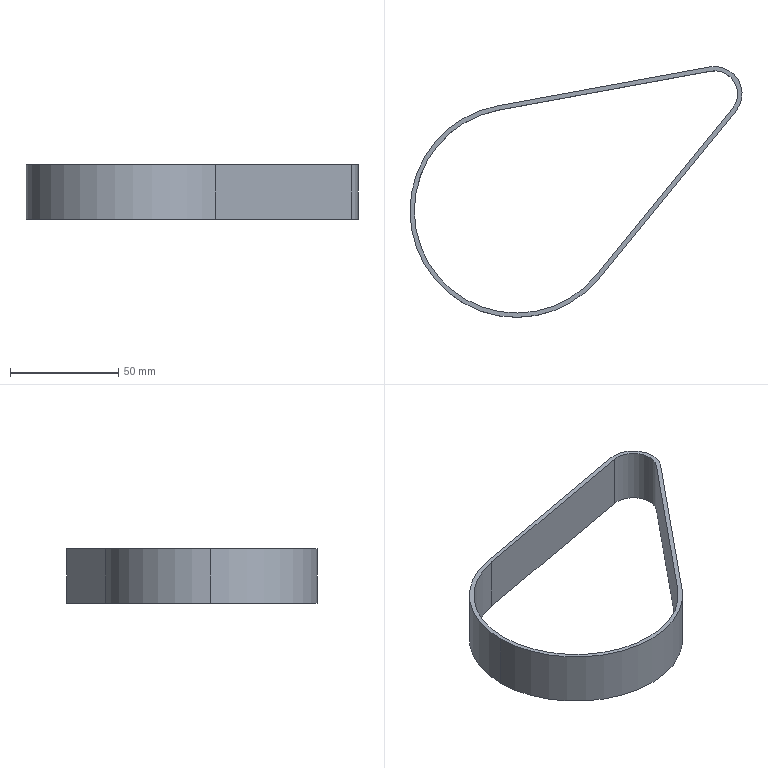Part | SolidWorks | features BaseBody 1 | 1 solid | 12 faces | box 153.425 x 115.925 x 25 mm | volume 20675 mm3 | plane 6 | cylinder 6 | commonest cylinder face diameters 94.53 x2 98.53 x2 21.32 x1 25.32 x1
STEP:
#1=CARTESIAN_POINT('',(-10.423,64.485,-12.5));
#2=VERTEX_POINT('',#1);
#3=CARTESIAN_POINT('',(-108.528,46.489,-12.5));
#4=VERTEX_POINT('',#3);
#5=CARTESIAN_POINT('',(-108.528,46.489,-12.5));
#6=DIRECTION('',(-0.9836,-0.1804,0.));
#7=VECTOR('',#6,1000.);
#8=LINE('',#5,#7);
#9=EDGE_CURVE('',#2,#4,#8,.T.);
#10=ORIENTED_EDGE('',*,*,#9,.F.);
#11=CARTESIAN_POINT('',(-10.423,64.485,12.5));
#12=VERTEX_POINT('',#11);
#13=CARTESIAN_POINT('',(-10.423,64.485,12.5));
#14=DIRECTION('',(0.,0.,-1.));
#15=VECTOR('',#14,1000.);
#16=LINE('',#13,#15);
#17=EDGE_CURVE('',#12,#2,#16,.T.);
#18=ORIENTED_EDGE('',*,*,#17,.F.);
#19=CARTESIAN_POINT('',(-108.528,46.489,12.5));
#20=VERTEX_POINT('',#19);
#21=CARTESIAN_POINT('',(-108.528,46.489,12.5));
#22=DIRECTION('',(-0.9836,-0.1804,0.));
#23=VECTOR('',#22,1000.);
#24=LINE('',#21,#23);
#25=EDGE_CURVE('',#12,#20,#24,.T.);
#26=ORIENTED_EDGE('',*,*,#25,.T.);
#27=CARTESIAN_POINT('',(-108.528,46.489,12.5));
#28=DIRECTION('',(0.,0.,-1.));
#29=VECTOR('',#28,1000.);
#30=LINE('',#27,#29);
#31=EDGE_CURVE('',#20,#4,#30,.T.);
#32=ORIENTED_EDGE('',*,*,#31,.T.);
#33=EDGE_LOOP('',(#10,#18,#26,#32));
#34=FACE_OUTER_BOUND('',#33,.T.);
#35=CARTESIAN_POINT('',(-108.528,46.489,12.5));
#36=DIRECTION('',(0.1804,-0.9836,0.));
#37=DIRECTION('',(0.,0.,-1.));
#38=AXIS2_PLACEMENT_3D('',#35,#36,#37);
#39=PLANE('',#38);
#40=ADVANCED_FACE('',(#34),#39,.T.);
#41=CARTESIAN_POINT('',(-0.2508,47.248,-12.5));
#42=VERTEX_POINT('',#41);
#43=CARTESIAN_POINT('',(-8.5,54.,-12.5));
#44=DIRECTION('',(0.,0.,1.));
#45=DIRECTION('',(-1.,0.,0.));
#46=AXIS2_PLACEMENT_3D('',#43,#44,#45);
#47=CIRCLE('',#46,10.66);
#48=EDGE_CURVE('',#42,#2,#47,.T.);
#49=ORIENTED_EDGE('',*,*,#48,.F.);
#50=CARTESIAN_POINT('',(-0.2508,47.248,12.5));
#51=VERTEX_POINT('',#50);
#52=CARTESIAN_POINT('',(-0.2508,47.248,12.5));
#53=DIRECTION('',(0.,0.,-1.));
#54=VECTOR('',#53,1000.);
#55=LINE('',#52,#54);
#56=EDGE_CURVE('',#51,#42,#55,.T.);
#57=ORIENTED_EDGE('',*,*,#56,.F.);
#58=CARTESIAN_POINT('',(-8.5,54.,12.5));
#59=DIRECTION('',(0.,0.,1.));
#60=DIRECTION('',(-1.,0.,0.));
#61=AXIS2_PLACEMENT_3D('',#58,#59,#60);
#62=CIRCLE('',#61,10.66);
#63=EDGE_CURVE('',#51,#12,#62,.T.);
#64=ORIENTED_EDGE('',*,*,#63,.T.);
#65=ORIENTED_EDGE('',*,*,#17,.T.);
#66=EDGE_LOOP('',(#49,#57,#64,#65));
#67=FACE_OUTER_BOUND('',#66,.T.);
#68=CARTESIAN_POINT('',(-8.5,54.,12.5));
#69=DIRECTION('',(0.,0.,-1.));
#70=DIRECTION('',(-1.,0.,0.));
#71=AXIS2_PLACEMENT_3D('',#68,#69,#70);
#72=CYLINDRICAL_SURFACE('',#71,10.66);
#73=ADVANCED_FACE('',(#67),#72,.F.);
#74=CARTESIAN_POINT('',(-63.424,-29.936,-12.5));
#75=VERTEX_POINT('',#74);
#76=CARTESIAN_POINT('',(-0.2508,47.248,-12.5));
#77=DIRECTION('',(0.6334,0.7738,0.));
#78=VECTOR('',#77,1000.);
#79=LINE('',#76,#78);
#80=EDGE_CURVE('',#75,#42,#79,.T.);
#81=ORIENTED_EDGE('',*,*,#80,.F.);
#82=CARTESIAN_POINT('',(-63.424,-29.936,12.5));
#83=VERTEX_POINT('',#82);
#84=CARTESIAN_POINT('',(-63.424,-29.936,12.5));
#85=DIRECTION('',(0.,0.,-1.));
#86=VECTOR('',#85,1000.);
#87=LINE('',#84,#86);
#88=EDGE_CURVE('',#83,#75,#87,.T.);
#89=ORIENTED_EDGE('',*,*,#88,.F.);
#90=CARTESIAN_POINT('',(-0.2508,47.248,12.5));
#91=DIRECTION('',(0.6334,0.7738,0.));
#92=VECTOR('',#91,1000.);
#93=LINE('',#90,#92);
#94=EDGE_CURVE('',#83,#51,#93,.T.);
#95=ORIENTED_EDGE('',*,*,#94,.T.);
#96=ORIENTED_EDGE('',*,*,#56,.T.);
#97=EDGE_LOOP('',(#81,#89,#95,#96));
#98=FACE_OUTER_BOUND('',#97,.T.);
#99=CARTESIAN_POINT('',(-0.2508,47.248,12.5));
#100=DIRECTION('',(-0.7738,0.6334,0.));
#101=DIRECTION('',(0.,0.,1.));
#102=AXIS2_PLACEMENT_3D('',#99,#100,#101);
#103=PLANE('',#102);
#104=ADVANCED_FACE('',(#98),#103,.T.);
#105=CARTESIAN_POINT('',(-147.265,0.,12.5));
#106=VERTEX_POINT('',#105);
#107=CARTESIAN_POINT('',(-147.265,0.,-12.5));
#108=VERTEX_POINT('',#107);
#109=CARTESIAN_POINT('',(-147.265,0.,12.5));
#110=DIRECTION('',(0.,0.,-1.));
#111=VECTOR('',#110,1000.);
#112=LINE('',#109,#111);
#113=EDGE_CURVE('',#106,#108,#112,.T.);
#114=ORIENTED_EDGE('',*,*,#113,.F.);
#115=CARTESIAN_POINT('',(-100.,0.,12.5));
#116=DIRECTION('',(0.,0.,1.));
#117=DIRECTION('',(-1.,0.,0.));
#118=AXIS2_PLACEMENT_3D('',#115,#116,#117);
#119=CIRCLE('',#118,47.265);
#120=EDGE_CURVE('',#106,#83,#119,.T.);
#121=ORIENTED_EDGE('',*,*,#120,.T.);
#122=ORIENTED_EDGE('',*,*,#88,.T.);
#123=CARTESIAN_POINT('',(-100.,0.,-12.5));
#124=DIRECTION('',(0.,0.,1.));
#125=DIRECTION('',(-1.,0.,0.));
#126=AXIS2_PLACEMENT_3D('',#123,#124,#125);
#127=CIRCLE('',#126,47.265);
#128=EDGE_CURVE('',#108,#75,#127,.T.);
#129=ORIENTED_EDGE('',*,*,#128,.F.);
#130=EDGE_LOOP('',(#114,#121,#122,#129));
#131=FACE_OUTER_BOUND('',#130,.T.);
#132=CARTESIAN_POINT('',(-100.,0.,12.5));
#133=DIRECTION('',(0.,0.,-1.));
#134=DIRECTION('',(-1.,0.,0.));
#135=AXIS2_PLACEMENT_3D('',#132,#133,#134);
#136=CYLINDRICAL_SURFACE('',#135,47.265);
#137=ADVANCED_FACE('',(#131),#136,.F.);
#138=CARTESIAN_POINT('',(-10.784,66.452,-12.5));
#139=VERTEX_POINT('',#138);
#140=CARTESIAN_POINT('',(-108.889,48.457,-12.5));
#141=VERTEX_POINT('',#140);
#142=CARTESIAN_POINT('',(-108.889,48.457,-12.5));
#143=DIRECTION('',(-0.9836,-0.1804,0.));
#144=VECTOR('',#143,1000.);
#145=LINE('',#142,#144);
#146=EDGE_CURVE('',#139,#141,#145,.T.);
#147=ORIENTED_EDGE('',*,*,#146,.T.);
#148=CARTESIAN_POINT('',(-108.889,48.457,12.5));
#149=VERTEX_POINT('',#148);
#150=CARTESIAN_POINT('',(-108.889,48.457,12.5));
#151=DIRECTION('',(0.,0.,-1.));
#152=VECTOR('',#151,1000.);
#153=LINE('',#150,#152);
#154=EDGE_CURVE('',#149,#141,#153,.T.);
#155=ORIENTED_EDGE('',*,*,#154,.F.);
#156=CARTESIAN_POINT('',(-10.784,66.452,12.5));
#157=VERTEX_POINT('',#156);
#158=CARTESIAN_POINT('',(-108.889,48.457,12.5));
#159=DIRECTION('',(-0.9836,-0.1804,0.));
#160=VECTOR('',#159,1000.);
#161=LINE('',#158,#160);
#162=EDGE_CURVE('',#157,#149,#161,.T.);
#163=ORIENTED_EDGE('',*,*,#162,.F.);
#164=CARTESIAN_POINT('',(-10.784,66.452,12.5));
#165=DIRECTION('',(0.,0.,-1.));
#166=VECTOR('',#165,1000.);
#167=LINE('',#164,#166);
#168=EDGE_CURVE('',#157,#139,#167,.T.);
#169=ORIENTED_EDGE('',*,*,#168,.T.);
#170=EDGE_LOOP('',(#147,#155,#163,#169));
#171=FACE_OUTER_BOUND('',#170,.T.);
#172=CARTESIAN_POINT('',(-108.889,48.457,12.5));
#173=DIRECTION('',(0.1804,-0.9836,0.));
#174=DIRECTION('',(0.,0.,-1.));
#175=AXIS2_PLACEMENT_3D('',#172,#173,#174);
#176=PLANE('',#175);
#177=ADVANCED_FACE('',(#171),#176,.F.);
#178=CARTESIAN_POINT('',(1.297,45.982,-12.5));
#179=VERTEX_POINT('',#178);
#180=CARTESIAN_POINT('',(-8.5,54.,-12.5));
#181=DIRECTION('',(0.,0.,1.));
#182=DIRECTION('',(-1.,0.,0.));
#183=AXIS2_PLACEMENT_3D('',#180,#181,#182);
#184=CIRCLE('',#183,12.66);
#185=EDGE_CURVE('',#179,#139,#184,.T.);
#186=ORIENTED_EDGE('',*,*,#185,.T.);
#187=ORIENTED_EDGE('',*,*,#168,.F.);
#188=CARTESIAN_POINT('',(1.297,45.982,12.5));
#189=VERTEX_POINT('',#188);
#190=CARTESIAN_POINT('',(-8.5,54.,12.5));
#191=DIRECTION('',(0.,0.,1.));
#192=DIRECTION('',(-1.,0.,0.));
#193=AXIS2_PLACEMENT_3D('',#190,#191,#192);
#194=CIRCLE('',#193,12.66);
#195=EDGE_CURVE('',#189,#157,#194,.T.);
#196=ORIENTED_EDGE('',*,*,#195,.F.);
#197=CARTESIAN_POINT('',(1.297,45.982,12.5));
#198=DIRECTION('',(0.,0.,-1.));
#199=VECTOR('',#198,1000.);
#200=LINE('',#197,#199);
#201=EDGE_CURVE('',#189,#179,#200,.T.);
#202=ORIENTED_EDGE('',*,*,#201,.T.);
#203=EDGE_LOOP('',(#186,#187,#196,#202));
#204=FACE_OUTER_BOUND('',#203,.T.);
#205=CARTESIAN_POINT('',(-8.5,54.,12.5));
#206=DIRECTION('',(0.,0.,-1.));
#207=DIRECTION('',(-1.,0.,0.));
#208=AXIS2_PLACEMENT_3D('',#205,#206,#207);
#209=CYLINDRICAL_SURFACE('',#208,12.66);
#210=ADVANCED_FACE('',(#204),#209,.T.);
#211=CARTESIAN_POINT('',(-61.876,-31.203,-12.5));
#212=VERTEX_POINT('',#211);
#213=CARTESIAN_POINT('',(-61.876,-31.203,-12.5));
#214=DIRECTION('',(0.6334,0.7738,0.));
#215=VECTOR('',#214,1000.);
#216=LINE('',#213,#215);
#217=EDGE_CURVE('',#212,#179,#216,.T.);
#218=ORIENTED_EDGE('',*,*,#217,.T.);
#219=ORIENTED_EDGE('',*,*,#201,.F.);
#220=CARTESIAN_POINT('',(-61.876,-31.203,12.5));
#221=VERTEX_POINT('',#220);
#222=CARTESIAN_POINT('',(-61.876,-31.203,12.5));
#223=DIRECTION('',(0.6334,0.7738,0.));
#224=VECTOR('',#223,1000.);
#225=LINE('',#222,#224);
#226=EDGE_CURVE('',#221,#189,#225,.T.);
#227=ORIENTED_EDGE('',*,*,#226,.F.);
#228=CARTESIAN_POINT('',(-61.876,-31.203,12.5));
#229=DIRECTION('',(0.,0.,-1.));
#230=VECTOR('',#229,1000.);
#231=LINE('',#228,#230);
#232=EDGE_CURVE('',#221,#212,#231,.T.);
#233=ORIENTED_EDGE('',*,*,#232,.T.);
#234=EDGE_LOOP('',(#218,#219,#227,#233));
#235=FACE_OUTER_BOUND('',#234,.T.);
#236=CARTESIAN_POINT('',(-61.876,-31.203,12.5));
#237=DIRECTION('',(-0.7738,0.6334,0.));
#238=DIRECTION('',(0.,0.,1.));
#239=AXIS2_PLACEMENT_3D('',#236,#237,#238);
#240=PLANE('',#239);
#241=ADVANCED_FACE('',(#235),#240,.F.);
#242=CARTESIAN_POINT('',(-149.265,0.,12.5));
#243=VERTEX_POINT('',#242);
#244=CARTESIAN_POINT('',(-149.265,0.,-12.5));
#245=VERTEX_POINT('',#244);
#246=CARTESIAN_POINT('',(-149.265,0.,12.5));
#247=DIRECTION('',(0.,0.,-1.));
#248=VECTOR('',#247,1000.);
#249=LINE('',#246,#248);
#250=EDGE_CURVE('',#243,#245,#249,.T.);
#251=ORIENTED_EDGE('',*,*,#250,.F.);
#252=CARTESIAN_POINT('',(-100.,0.,12.5));
#253=DIRECTION('',(0.,0.,1.));
#254=DIRECTION('',(-1.,0.,0.));
#255=AXIS2_PLACEMENT_3D('',#252,#253,#254);
#256=CIRCLE('',#255,49.265);
#257=EDGE_CURVE('',#149,#243,#256,.T.);
#258=ORIENTED_EDGE('',*,*,#257,.F.);
#259=ORIENTED_EDGE('',*,*,#154,.T.);
#260=CARTESIAN_POINT('',(-100.,0.,-12.5));
#261=DIRECTION('',(0.,0.,1.));
#262=DIRECTION('',(-1.,0.,0.));
#263=AXIS2_PLACEMENT_3D('',#260,#261,#262);
#264=CIRCLE('',#263,49.265);
#265=EDGE_CURVE('',#141,#245,#264,.T.);
#266=ORIENTED_EDGE('',*,*,#265,.T.);
#267=EDGE_LOOP('',(#251,#258,#259,#266));
#268=FACE_OUTER_BOUND('',#267,.T.);
#269=CARTESIAN_POINT('',(-100.,0.,12.5));
#270=DIRECTION('',(0.,0.,-1.));
#271=DIRECTION('',(-1.,0.,0.));
#272=AXIS2_PLACEMENT_3D('',#269,#270,#271);
#273=CYLINDRICAL_SURFACE('',#272,49.265);
#274=ADVANCED_FACE('',(#268),#273,.T.);
#275=ORIENTED_EDGE('',*,*,#9,.T.);
#276=CARTESIAN_POINT('',(-100.,0.,-12.5));
#277=DIRECTION('',(0.,0.,1.));
#278=DIRECTION('',(-1.,0.,0.));
#279=AXIS2_PLACEMENT_3D('',#276,#277,#278);
#280=CIRCLE('',#279,47.265);
#281=EDGE_CURVE('',#4,#108,#280,.T.);
#282=ORIENTED_EDGE('',*,*,#281,.T.);
#283=ORIENTED_EDGE('',*,*,#128,.T.);
#284=ORIENTED_EDGE('',*,*,#80,.T.);
#285=ORIENTED_EDGE('',*,*,#48,.T.);
#286=EDGE_LOOP('',(#275,#282,#283,#284,#285));
#287=FACE_BOUND('',#286,.T.);
#288=ORIENTED_EDGE('',*,*,#265,.F.);
#289=ORIENTED_EDGE('',*,*,#146,.F.);
#290=ORIENTED_EDGE('',*,*,#185,.F.);
#291=ORIENTED_EDGE('',*,*,#217,.F.);
#292=CARTESIAN_POINT('',(-100.,0.,-12.5));
#293=DIRECTION('',(0.,0.,1.));
#294=DIRECTION('',(-1.,0.,0.));
#295=AXIS2_PLACEMENT_3D('',#292,#293,#294);
#296=CIRCLE('',#295,49.265);
#297=EDGE_CURVE('',#245,#212,#296,.T.);
#298=ORIENTED_EDGE('',*,*,#297,.F.);
#299=EDGE_LOOP('',(#288,#289,#290,#291,#298));
#300=FACE_OUTER_BOUND('',#299,.T.);
#301=CARTESIAN_POINT('',(-100.,0.,-12.5));
#302=DIRECTION('',(0.,0.,-1.));
#303=DIRECTION('',(0.,-1.,0.));
#304=AXIS2_PLACEMENT_3D('',#301,#302,#303);
#305=PLANE('',#304);
#306=ADVANCED_FACE('',(#287,#300),#305,.T.);
#307=CARTESIAN_POINT('',(-100.,0.,12.5));
#308=DIRECTION('',(0.,0.,1.));
#309=DIRECTION('',(-1.,0.,0.));
#310=AXIS2_PLACEMENT_3D('',#307,#308,#309);
#311=CIRCLE('',#310,47.265);
#312=EDGE_CURVE('',#20,#106,#311,.T.);
#313=ORIENTED_EDGE('',*,*,#312,.F.);
#314=ORIENTED_EDGE('',*,*,#25,.F.);
#315=ORIENTED_EDGE('',*,*,#63,.F.);
#316=ORIENTED_EDGE('',*,*,#94,.F.);
#317=ORIENTED_EDGE('',*,*,#120,.F.);
#318=EDGE_LOOP('',(#313,#314,#315,#316,#317));
#319=FACE_BOUND('',#318,.T.);
#320=ORIENTED_EDGE('',*,*,#257,.T.);
#321=CARTESIAN_POINT('',(-100.,0.,12.5));
#322=DIRECTION('',(0.,0.,1.));
#323=DIRECTION('',(-1.,0.,0.));
#324=AXIS2_PLACEMENT_3D('',#321,#322,#323);
#325=CIRCLE('',#324,49.265);
#326=EDGE_CURVE('',#243,#221,#325,.T.);
#327=ORIENTED_EDGE('',*,*,#326,.T.);
#328=ORIENTED_EDGE('',*,*,#226,.T.);
#329=ORIENTED_EDGE('',*,*,#195,.T.);
#330=ORIENTED_EDGE('',*,*,#162,.T.);
#331=EDGE_LOOP('',(#320,#327,#328,#329,#330));
#332=FACE_OUTER_BOUND('',#331,.T.);
#333=CARTESIAN_POINT('',(-100.,0.,12.5));
#334=DIRECTION('',(0.,0.,-1.));
#335=DIRECTION('',(0.,-1.,0.));
#336=AXIS2_PLACEMENT_3D('',#333,#334,#335);
#337=PLANE('',#336);
#338=ADVANCED_FACE('',(#319,#332),#337,.F.);
#339=ORIENTED_EDGE('',*,*,#326,.F.);
#340=ORIENTED_EDGE('',*,*,#250,.T.);
#341=ORIENTED_EDGE('',*,*,#297,.T.);
#342=ORIENTED_EDGE('',*,*,#232,.F.);
#343=EDGE_LOOP('',(#339,#340,#341,#342));
#344=FACE_OUTER_BOUND('',#343,.T.);
#345=CARTESIAN_POINT('',(-100.,0.,12.5));
#346=DIRECTION('',(0.,0.,-1.));
#347=DIRECTION('',(-1.,0.,0.));
#348=AXIS2_PLACEMENT_3D('',#345,#346,#347);
#349=CYLINDRICAL_SURFACE('',#348,49.265);
#350=ADVANCED_FACE('',(#344),#349,.T.);
#351=ORIENTED_EDGE('',*,*,#312,.T.);
#352=ORIENTED_EDGE('',*,*,#113,.T.);
#353=ORIENTED_EDGE('',*,*,#281,.F.);
#354=ORIENTED_EDGE('',*,*,#31,.F.);
#355=EDGE_LOOP('',(#351,#352,#353,#354));
#356=FACE_OUTER_BOUND('',#355,.T.);
#357=CARTESIAN_POINT('',(-100.,0.,12.5));
#358=DIRECTION('',(0.,0.,-1.));
#359=DIRECTION('',(-1.,0.,0.));
#360=AXIS2_PLACEMENT_3D('',#357,#358,#359);
#361=CYLINDRICAL_SURFACE('',#360,47.265);
#362=ADVANCED_FACE('',(#356),#361,.F.);
#363=CLOSED_SHELL('',(#40,#73,#104,#137,#177,#210,#241,#274,#306,#338,#350,#362));
#364=MANIFOLD_SOLID_BREP('',#363);
#365=CARTESIAN_POINT('',(0.,0.,0.));
#366=DIRECTION('',(0.,0.,1.));
#367=DIRECTION('',(1.,0.,0.));
#368=AXIS2_PLACEMENT_3D('',#365,#366,#367);
#369=(LENGTH_UNIT()NAMED_UNIT(*)SI_UNIT(.MILLI.,.METRE.));
#370=UNCERTAINTY_MEASURE_WITH_UNIT(LENGTH_MEASURE(0.00001),#369,'','');
#371=(NAMED_UNIT(*)PLANE_ANGLE_UNIT()SI_UNIT($,.RADIAN.));
#372=(NAMED_UNIT(*)SI_UNIT($,.STERADIAN.)SOLID_ANGLE_UNIT());
#373=(GEOMETRIC_REPRESENTATION_CONTEXT(3)GLOBAL_UNCERTAINTY_ASSIGNED_CONTEXT((#370))GLOBAL_UNIT_ASSIGNED_CONTEXT((#369,#371,#372))REPRESENTATION_CONTEXT('',''));
#374=ADVANCED_BREP_SHAPE_REPRESENTATION('',(#364,#368),#373);